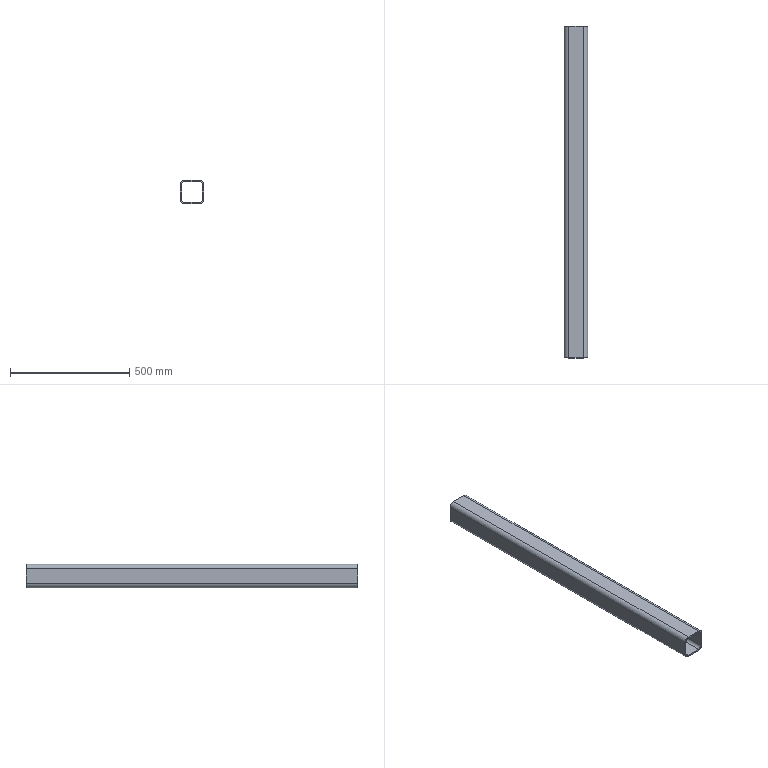Part | SolidWorks | features WeldMemberFeat 1, WeldmentFeature 1 | 1 solid | 18 faces | box 100 x 1393 x 100 mm | volume 2912161 mm3 | plane 10 | cylinder 8 | commonest cylinder face diameters 26.12 x4 38.12 x4
STEP:
#1=CARTESIAN_POINT('',(-50.,0.,30.94));
#2=VERTEX_POINT('',#1);
#3=CARTESIAN_POINT('',(-30.94,0.,50.));
#4=VERTEX_POINT('',#3);
#5=CARTESIAN_POINT('',(-30.94,0.,30.94));
#6=DIRECTION('',(0.,1.,0.));
#7=DIRECTION('',(0.,0.,1.));
#8=AXIS2_PLACEMENT_3D('',#5,#6,#7);
#9=CIRCLE('',#8,19.06);
#10=EDGE_CURVE('',#2,#4,#9,.T.);
#11=ORIENTED_EDGE('',*,*,#10,.T.);
#12=CARTESIAN_POINT('',(-30.94,1393.,50.));
#13=VERTEX_POINT('',#12);
#14=CARTESIAN_POINT('',(-30.94,1393.,50.));
#15=DIRECTION('',(0.,-1.,0.));
#16=VECTOR('',#15,1000.);
#17=LINE('',#14,#16);
#18=EDGE_CURVE('',#13,#4,#17,.T.);
#19=ORIENTED_EDGE('',*,*,#18,.F.);
#20=CARTESIAN_POINT('',(-50.,1393.,30.94));
#21=VERTEX_POINT('',#20);
#22=CARTESIAN_POINT('',(-30.94,1393.,30.94));
#23=DIRECTION('',(0.,1.,0.));
#24=DIRECTION('',(0.,0.,1.));
#25=AXIS2_PLACEMENT_3D('',#22,#23,#24);
#26=CIRCLE('',#25,19.06);
#27=EDGE_CURVE('',#21,#13,#26,.T.);
#28=ORIENTED_EDGE('',*,*,#27,.F.);
#29=CARTESIAN_POINT('',(-50.,1393.,30.94));
#30=DIRECTION('',(0.,-1.,0.));
#31=VECTOR('',#30,1000.);
#32=LINE('',#29,#31);
#33=EDGE_CURVE('',#21,#2,#32,.T.);
#34=ORIENTED_EDGE('',*,*,#33,.T.);
#35=EDGE_LOOP('',(#11,#19,#28,#34));
#36=FACE_OUTER_BOUND('',#35,.T.);
#37=CARTESIAN_POINT('',(-30.94,1393.,30.94));
#38=DIRECTION('',(0.,-1.,0.));
#39=DIRECTION('',(0.,0.,-1.));
#40=AXIS2_PLACEMENT_3D('',#37,#38,#39);
#41=CYLINDRICAL_SURFACE('',#40,19.06);
#42=ADVANCED_FACE('',(#36),#41,.T.);
#43=CARTESIAN_POINT('',(30.94,0.,50.));
#44=VERTEX_POINT('',#43);
#45=CARTESIAN_POINT('',(-30.94,0.,50.));
#46=DIRECTION('',(1.,0.,0.));
#47=VECTOR('',#46,1000.);
#48=LINE('',#45,#47);
#49=EDGE_CURVE('',#4,#44,#48,.T.);
#50=ORIENTED_EDGE('',*,*,#49,.T.);
#51=CARTESIAN_POINT('',(30.94,1393.,50.));
#52=VERTEX_POINT('',#51);
#53=CARTESIAN_POINT('',(30.94,1393.,50.));
#54=DIRECTION('',(0.,-1.,0.));
#55=VECTOR('',#54,1000.);
#56=LINE('',#53,#55);
#57=EDGE_CURVE('',#52,#44,#56,.T.);
#58=ORIENTED_EDGE('',*,*,#57,.F.);
#59=CARTESIAN_POINT('',(-30.94,1393.,50.));
#60=DIRECTION('',(1.,0.,0.));
#61=VECTOR('',#60,1000.);
#62=LINE('',#59,#61);
#63=EDGE_CURVE('',#13,#52,#62,.T.);
#64=ORIENTED_EDGE('',*,*,#63,.F.);
#65=ORIENTED_EDGE('',*,*,#18,.T.);
#66=EDGE_LOOP('',(#50,#58,#64,#65));
#67=FACE_OUTER_BOUND('',#66,.T.);
#68=CARTESIAN_POINT('',(-30.94,1393.,50.));
#69=DIRECTION('',(0.,0.,-1.));
#70=DIRECTION('',(-1.,0.,0.));
#71=AXIS2_PLACEMENT_3D('',#68,#69,#70);
#72=PLANE('',#71);
#73=ADVANCED_FACE('',(#67),#72,.F.);
#74=CARTESIAN_POINT('',(50.,0.,30.94));
#75=VERTEX_POINT('',#74);
#76=CARTESIAN_POINT('',(30.94,0.,30.94));
#77=DIRECTION('',(0.,1.,0.));
#78=DIRECTION('',(0.,0.,1.));
#79=AXIS2_PLACEMENT_3D('',#76,#77,#78);
#80=CIRCLE('',#79,19.06);
#81=EDGE_CURVE('',#44,#75,#80,.T.);
#82=ORIENTED_EDGE('',*,*,#81,.T.);
#83=CARTESIAN_POINT('',(50.,1393.,30.94));
#84=VERTEX_POINT('',#83);
#85=CARTESIAN_POINT('',(50.,1393.,30.94));
#86=DIRECTION('',(0.,-1.,0.));
#87=VECTOR('',#86,1000.);
#88=LINE('',#85,#87);
#89=EDGE_CURVE('',#84,#75,#88,.T.);
#90=ORIENTED_EDGE('',*,*,#89,.F.);
#91=CARTESIAN_POINT('',(30.94,1393.,30.94));
#92=DIRECTION('',(0.,1.,0.));
#93=DIRECTION('',(0.,0.,1.));
#94=AXIS2_PLACEMENT_3D('',#91,#92,#93);
#95=CIRCLE('',#94,19.06);
#96=EDGE_CURVE('',#52,#84,#95,.T.);
#97=ORIENTED_EDGE('',*,*,#96,.F.);
#98=ORIENTED_EDGE('',*,*,#57,.T.);
#99=EDGE_LOOP('',(#82,#90,#97,#98));
#100=FACE_OUTER_BOUND('',#99,.T.);
#101=CARTESIAN_POINT('',(30.94,1393.,30.94));
#102=DIRECTION('',(0.,-1.,0.));
#103=DIRECTION('',(0.,0.,-1.));
#104=AXIS2_PLACEMENT_3D('',#101,#102,#103);
#105=CYLINDRICAL_SURFACE('',#104,19.06);
#106=ADVANCED_FACE('',(#100),#105,.T.);
#107=CARTESIAN_POINT('',(50.,0.,-30.94));
#108=VERTEX_POINT('',#107);
#109=CARTESIAN_POINT('',(50.,0.,-30.94));
#110=DIRECTION('',(0.,0.,-1.));
#111=VECTOR('',#110,1000.);
#112=LINE('',#109,#111);
#113=EDGE_CURVE('',#75,#108,#112,.T.);
#114=ORIENTED_EDGE('',*,*,#113,.T.);
#115=CARTESIAN_POINT('',(50.,1393.,-30.94));
#116=VERTEX_POINT('',#115);
#117=CARTESIAN_POINT('',(50.,1393.,-30.94));
#118=DIRECTION('',(0.,-1.,0.));
#119=VECTOR('',#118,1000.);
#120=LINE('',#117,#119);
#121=EDGE_CURVE('',#116,#108,#120,.T.);
#122=ORIENTED_EDGE('',*,*,#121,.F.);
#123=CARTESIAN_POINT('',(50.,1393.,-30.94));
#124=DIRECTION('',(0.,0.,-1.));
#125=VECTOR('',#124,1000.);
#126=LINE('',#123,#125);
#127=EDGE_CURVE('',#84,#116,#126,.T.);
#128=ORIENTED_EDGE('',*,*,#127,.F.);
#129=ORIENTED_EDGE('',*,*,#89,.T.);
#130=EDGE_LOOP('',(#114,#122,#128,#129));
#131=FACE_OUTER_BOUND('',#130,.T.);
#132=CARTESIAN_POINT('',(50.,1393.,-30.94));
#133=DIRECTION('',(-1.,0.,0.));
#134=DIRECTION('',(0.,0.,1.));
#135=AXIS2_PLACEMENT_3D('',#132,#133,#134);
#136=PLANE('',#135);
#137=ADVANCED_FACE('',(#131),#136,.F.);
#138=CARTESIAN_POINT('',(30.94,0.,-50.));
#139=VERTEX_POINT('',#138);
#140=CARTESIAN_POINT('',(30.94,0.,-30.94));
#141=DIRECTION('',(0.,1.,0.));
#142=DIRECTION('',(0.,0.,1.));
#143=AXIS2_PLACEMENT_3D('',#140,#141,#142);
#144=CIRCLE('',#143,19.06);
#145=EDGE_CURVE('',#108,#139,#144,.T.);
#146=ORIENTED_EDGE('',*,*,#145,.T.);
#147=CARTESIAN_POINT('',(30.94,1393.,-50.));
#148=VERTEX_POINT('',#147);
#149=CARTESIAN_POINT('',(30.94,1393.,-50.));
#150=DIRECTION('',(0.,-1.,0.));
#151=VECTOR('',#150,1000.);
#152=LINE('',#149,#151);
#153=EDGE_CURVE('',#148,#139,#152,.T.);
#154=ORIENTED_EDGE('',*,*,#153,.F.);
#155=CARTESIAN_POINT('',(30.94,1393.,-30.94));
#156=DIRECTION('',(0.,1.,0.));
#157=DIRECTION('',(0.,0.,1.));
#158=AXIS2_PLACEMENT_3D('',#155,#156,#157);
#159=CIRCLE('',#158,19.06);
#160=EDGE_CURVE('',#116,#148,#159,.T.);
#161=ORIENTED_EDGE('',*,*,#160,.F.);
#162=ORIENTED_EDGE('',*,*,#121,.T.);
#163=EDGE_LOOP('',(#146,#154,#161,#162));
#164=FACE_OUTER_BOUND('',#163,.T.);
#165=CARTESIAN_POINT('',(30.94,1393.,-30.94));
#166=DIRECTION('',(0.,-1.,0.));
#167=DIRECTION('',(0.,0.,-1.));
#168=AXIS2_PLACEMENT_3D('',#165,#166,#167);
#169=CYLINDRICAL_SURFACE('',#168,19.06);
#170=ADVANCED_FACE('',(#164),#169,.T.);
#171=CARTESIAN_POINT('',(-30.94,0.,-50.));
#172=VERTEX_POINT('',#171);
#173=CARTESIAN_POINT('',(30.94,0.,-50.));
#174=DIRECTION('',(-1.,0.,0.));
#175=VECTOR('',#174,1000.);
#176=LINE('',#173,#175);
#177=EDGE_CURVE('',#139,#172,#176,.T.);
#178=ORIENTED_EDGE('',*,*,#177,.T.);
#179=CARTESIAN_POINT('',(-30.94,1393.,-50.));
#180=VERTEX_POINT('',#179);
#181=CARTESIAN_POINT('',(-30.94,1393.,-50.));
#182=DIRECTION('',(0.,-1.,0.));
#183=VECTOR('',#182,1000.);
#184=LINE('',#181,#183);
#185=EDGE_CURVE('',#180,#172,#184,.T.);
#186=ORIENTED_EDGE('',*,*,#185,.F.);
#187=CARTESIAN_POINT('',(30.94,1393.,-50.));
#188=DIRECTION('',(-1.,0.,0.));
#189=VECTOR('',#188,1000.);
#190=LINE('',#187,#189);
#191=EDGE_CURVE('',#148,#180,#190,.T.);
#192=ORIENTED_EDGE('',*,*,#191,.F.);
#193=ORIENTED_EDGE('',*,*,#153,.T.);
#194=EDGE_LOOP('',(#178,#186,#192,#193));
#195=FACE_OUTER_BOUND('',#194,.T.);
#196=CARTESIAN_POINT('',(30.94,1393.,-50.));
#197=DIRECTION('',(0.,0.,1.));
#198=DIRECTION('',(1.,0.,0.));
#199=AXIS2_PLACEMENT_3D('',#196,#197,#198);
#200=PLANE('',#199);
#201=ADVANCED_FACE('',(#195),#200,.F.);
#202=CARTESIAN_POINT('',(-50.,0.,-30.94));
#203=VERTEX_POINT('',#202);
#204=CARTESIAN_POINT('',(-30.94,0.,-30.94));
#205=DIRECTION('',(0.,1.,0.));
#206=DIRECTION('',(0.,0.,1.));
#207=AXIS2_PLACEMENT_3D('',#204,#205,#206);
#208=CIRCLE('',#207,19.06);
#209=EDGE_CURVE('',#172,#203,#208,.T.);
#210=ORIENTED_EDGE('',*,*,#209,.T.);
#211=CARTESIAN_POINT('',(-50.,1393.,-30.94));
#212=VERTEX_POINT('',#211);
#213=CARTESIAN_POINT('',(-50.,1393.,-30.94));
#214=DIRECTION('',(0.,-1.,0.));
#215=VECTOR('',#214,1000.);
#216=LINE('',#213,#215);
#217=EDGE_CURVE('',#212,#203,#216,.T.);
#218=ORIENTED_EDGE('',*,*,#217,.F.);
#219=CARTESIAN_POINT('',(-30.94,1393.,-30.94));
#220=DIRECTION('',(0.,1.,0.));
#221=DIRECTION('',(0.,0.,1.));
#222=AXIS2_PLACEMENT_3D('',#219,#220,#221);
#223=CIRCLE('',#222,19.06);
#224=EDGE_CURVE('',#180,#212,#223,.T.);
#225=ORIENTED_EDGE('',*,*,#224,.F.);
#226=ORIENTED_EDGE('',*,*,#185,.T.);
#227=EDGE_LOOP('',(#210,#218,#225,#226));
#228=FACE_OUTER_BOUND('',#227,.T.);
#229=CARTESIAN_POINT('',(-30.94,1393.,-30.94));
#230=DIRECTION('',(0.,-1.,0.));
#231=DIRECTION('',(0.,0.,-1.));
#232=AXIS2_PLACEMENT_3D('',#229,#230,#231);
#233=CYLINDRICAL_SURFACE('',#232,19.06);
#234=ADVANCED_FACE('',(#228),#233,.T.);
#235=CARTESIAN_POINT('',(30.94,0.,44.));
#236=VERTEX_POINT('',#235);
#237=CARTESIAN_POINT('',(44.,0.,30.94));
#238=VERTEX_POINT('',#237);
#239=CARTESIAN_POINT('',(30.94,0.,30.94));
#240=DIRECTION('',(0.,1.,0.));
#241=DIRECTION('',(0.,0.,1.));
#242=AXIS2_PLACEMENT_3D('',#239,#240,#241);
#243=CIRCLE('',#242,13.06);
#244=EDGE_CURVE('',#236,#238,#243,.T.);
#245=ORIENTED_EDGE('',*,*,#244,.F.);
#246=CARTESIAN_POINT('',(30.94,1393.,44.));
#247=VERTEX_POINT('',#246);
#248=CARTESIAN_POINT('',(30.94,1393.,44.));
#249=DIRECTION('',(0.,-1.,0.));
#250=VECTOR('',#249,1000.);
#251=LINE('',#248,#250);
#252=EDGE_CURVE('',#247,#236,#251,.T.);
#253=ORIENTED_EDGE('',*,*,#252,.F.);
#254=CARTESIAN_POINT('',(44.,1393.,30.94));
#255=VERTEX_POINT('',#254);
#256=CARTESIAN_POINT('',(30.94,1393.,30.94));
#257=DIRECTION('',(0.,1.,0.));
#258=DIRECTION('',(0.,0.,1.));
#259=AXIS2_PLACEMENT_3D('',#256,#257,#258);
#260=CIRCLE('',#259,13.06);
#261=EDGE_CURVE('',#247,#255,#260,.T.);
#262=ORIENTED_EDGE('',*,*,#261,.T.);
#263=CARTESIAN_POINT('',(44.,1393.,30.94));
#264=DIRECTION('',(0.,-1.,0.));
#265=VECTOR('',#264,1000.);
#266=LINE('',#263,#265);
#267=EDGE_CURVE('',#255,#238,#266,.T.);
#268=ORIENTED_EDGE('',*,*,#267,.T.);
#269=EDGE_LOOP('',(#245,#253,#262,#268));
#270=FACE_OUTER_BOUND('',#269,.T.);
#271=CARTESIAN_POINT('',(30.94,1393.,30.94));
#272=DIRECTION('',(0.,-1.,0.));
#273=DIRECTION('',(0.,0.,-1.));
#274=AXIS2_PLACEMENT_3D('',#271,#272,#273);
#275=CYLINDRICAL_SURFACE('',#274,13.06);
#276=ADVANCED_FACE('',(#270),#275,.F.);
#277=CARTESIAN_POINT('',(-30.94,0.,44.));
#278=VERTEX_POINT('',#277);
#279=CARTESIAN_POINT('',(-30.94,0.,44.));
#280=DIRECTION('',(1.,0.,0.));
#281=VECTOR('',#280,1000.);
#282=LINE('',#279,#281);
#283=EDGE_CURVE('',#278,#236,#282,.T.);
#284=ORIENTED_EDGE('',*,*,#283,.F.);
#285=CARTESIAN_POINT('',(-30.94,1393.,44.));
#286=VERTEX_POINT('',#285);
#287=CARTESIAN_POINT('',(-30.94,1393.,44.));
#288=DIRECTION('',(0.,-1.,0.));
#289=VECTOR('',#288,1000.);
#290=LINE('',#287,#289);
#291=EDGE_CURVE('',#286,#278,#290,.T.);
#292=ORIENTED_EDGE('',*,*,#291,.F.);
#293=CARTESIAN_POINT('',(-30.94,1393.,44.));
#294=DIRECTION('',(1.,0.,0.));
#295=VECTOR('',#294,1000.);
#296=LINE('',#293,#295);
#297=EDGE_CURVE('',#286,#247,#296,.T.);
#298=ORIENTED_EDGE('',*,*,#297,.T.);
#299=ORIENTED_EDGE('',*,*,#252,.T.);
#300=EDGE_LOOP('',(#284,#292,#298,#299));
#301=FACE_OUTER_BOUND('',#300,.T.);
#302=CARTESIAN_POINT('',(-30.94,1393.,44.));
#303=DIRECTION('',(0.,0.,-1.));
#304=DIRECTION('',(-1.,0.,0.));
#305=AXIS2_PLACEMENT_3D('',#302,#303,#304);
#306=PLANE('',#305);
#307=ADVANCED_FACE('',(#301),#306,.T.);
#308=CARTESIAN_POINT('',(-44.,0.,30.94));
#309=VERTEX_POINT('',#308);
#310=CARTESIAN_POINT('',(-30.94,0.,30.94));
#311=DIRECTION('',(0.,1.,0.));
#312=DIRECTION('',(0.,0.,1.));
#313=AXIS2_PLACEMENT_3D('',#310,#311,#312);
#314=CIRCLE('',#313,13.06);
#315=EDGE_CURVE('',#309,#278,#314,.T.);
#316=ORIENTED_EDGE('',*,*,#315,.F.);
#317=CARTESIAN_POINT('',(-44.,1393.,30.94));
#318=VERTEX_POINT('',#317);
#319=CARTESIAN_POINT('',(-44.,1393.,30.94));
#320=DIRECTION('',(0.,-1.,0.));
#321=VECTOR('',#320,1000.);
#322=LINE('',#319,#321);
#323=EDGE_CURVE('',#318,#309,#322,.T.);
#324=ORIENTED_EDGE('',*,*,#323,.F.);
#325=CARTESIAN_POINT('',(-30.94,1393.,30.94));
#326=DIRECTION('',(0.,1.,0.));
#327=DIRECTION('',(0.,0.,1.));
#328=AXIS2_PLACEMENT_3D('',#325,#326,#327);
#329=CIRCLE('',#328,13.06);
#330=EDGE_CURVE('',#318,#286,#329,.T.);
#331=ORIENTED_EDGE('',*,*,#330,.T.);
#332=ORIENTED_EDGE('',*,*,#291,.T.);
#333=EDGE_LOOP('',(#316,#324,#331,#332));
#334=FACE_OUTER_BOUND('',#333,.T.);
#335=CARTESIAN_POINT('',(-30.94,1393.,30.94));
#336=DIRECTION('',(0.,-1.,0.));
#337=DIRECTION('',(0.,0.,-1.));
#338=AXIS2_PLACEMENT_3D('',#335,#336,#337);
#339=CYLINDRICAL_SURFACE('',#338,13.06);
#340=ADVANCED_FACE('',(#334),#339,.F.);
#341=CARTESIAN_POINT('',(-44.,0.,-30.94));
#342=VERTEX_POINT('',#341);
#343=CARTESIAN_POINT('',(-44.,0.,30.94));
#344=DIRECTION('',(0.,0.,1.));
#345=VECTOR('',#344,1000.);
#346=LINE('',#343,#345);
#347=EDGE_CURVE('',#342,#309,#346,.T.);
#348=ORIENTED_EDGE('',*,*,#347,.F.);
#349=CARTESIAN_POINT('',(-44.,1393.,-30.94));
#350=VERTEX_POINT('',#349);
#351=CARTESIAN_POINT('',(-44.,1393.,-30.94));
#352=DIRECTION('',(0.,-1.,0.));
#353=VECTOR('',#352,1000.);
#354=LINE('',#351,#353);
#355=EDGE_CURVE('',#350,#342,#354,.T.);
#356=ORIENTED_EDGE('',*,*,#355,.F.);
#357=CARTESIAN_POINT('',(-44.,1393.,30.94));
#358=DIRECTION('',(0.,0.,1.));
#359=VECTOR('',#358,1000.);
#360=LINE('',#357,#359);
#361=EDGE_CURVE('',#350,#318,#360,.T.);
#362=ORIENTED_EDGE('',*,*,#361,.T.);
#363=ORIENTED_EDGE('',*,*,#323,.T.);
#364=EDGE_LOOP('',(#348,#356,#362,#363));
#365=FACE_OUTER_BOUND('',#364,.T.);
#366=CARTESIAN_POINT('',(-44.,1393.,30.94));
#367=DIRECTION('',(1.,0.,0.));
#368=DIRECTION('',(0.,0.,-1.));
#369=AXIS2_PLACEMENT_3D('',#366,#367,#368);
#370=PLANE('',#369);
#371=ADVANCED_FACE('',(#365),#370,.T.);
#372=CARTESIAN_POINT('',(-30.94,0.,-44.));
#373=VERTEX_POINT('',#372);
#374=CARTESIAN_POINT('',(-30.94,0.,-30.94));
#375=DIRECTION('',(0.,1.,0.));
#376=DIRECTION('',(0.,0.,1.));
#377=AXIS2_PLACEMENT_3D('',#374,#375,#376);
#378=CIRCLE('',#377,13.06);
#379=EDGE_CURVE('',#373,#342,#378,.T.);
#380=ORIENTED_EDGE('',*,*,#379,.F.);
#381=CARTESIAN_POINT('',(-30.94,1393.,-44.));
#382=VERTEX_POINT('',#381);
#383=CARTESIAN_POINT('',(-30.94,1393.,-44.));
#384=DIRECTION('',(0.,-1.,0.));
#385=VECTOR('',#384,1000.);
#386=LINE('',#383,#385);
#387=EDGE_CURVE('',#382,#373,#386,.T.);
#388=ORIENTED_EDGE('',*,*,#387,.F.);
#389=CARTESIAN_POINT('',(-30.94,1393.,-30.94));
#390=DIRECTION('',(0.,1.,0.));
#391=DIRECTION('',(0.,0.,1.));
#392=AXIS2_PLACEMENT_3D('',#389,#390,#391);
#393=CIRCLE('',#392,13.06);
#394=EDGE_CURVE('',#382,#350,#393,.T.);
#395=ORIENTED_EDGE('',*,*,#394,.T.);
#396=ORIENTED_EDGE('',*,*,#355,.T.);
#397=EDGE_LOOP('',(#380,#388,#395,#396));
#398=FACE_OUTER_BOUND('',#397,.T.);
#399=CARTESIAN_POINT('',(-30.94,1393.,-30.94));
#400=DIRECTION('',(0.,-1.,0.));
#401=DIRECTION('',(0.,0.,-1.));
#402=AXIS2_PLACEMENT_3D('',#399,#400,#401);
#403=CYLINDRICAL_SURFACE('',#402,13.06);
#404=ADVANCED_FACE('',(#398),#403,.F.);
#405=CARTESIAN_POINT('',(30.94,0.,-44.));
#406=VERTEX_POINT('',#405);
#407=CARTESIAN_POINT('',(30.94,0.,-44.));
#408=DIRECTION('',(-1.,0.,0.));
#409=VECTOR('',#408,1000.);
#410=LINE('',#407,#409);
#411=EDGE_CURVE('',#406,#373,#410,.T.);
#412=ORIENTED_EDGE('',*,*,#411,.F.);
#413=CARTESIAN_POINT('',(30.94,1393.,-44.));
#414=VERTEX_POINT('',#413);
#415=CARTESIAN_POINT('',(30.94,1393.,-44.));
#416=DIRECTION('',(0.,-1.,0.));
#417=VECTOR('',#416,1000.);
#418=LINE('',#415,#417);
#419=EDGE_CURVE('',#414,#406,#418,.T.);
#420=ORIENTED_EDGE('',*,*,#419,.F.);
#421=CARTESIAN_POINT('',(30.94,1393.,-44.));
#422=DIRECTION('',(-1.,0.,0.));
#423=VECTOR('',#422,1000.);
#424=LINE('',#421,#423);
#425=EDGE_CURVE('',#414,#382,#424,.T.);
#426=ORIENTED_EDGE('',*,*,#425,.T.);
#427=ORIENTED_EDGE('',*,*,#387,.T.);
#428=EDGE_LOOP('',(#412,#420,#426,#427));
#429=FACE_OUTER_BOUND('',#428,.T.);
#430=CARTESIAN_POINT('',(30.94,1393.,-44.));
#431=DIRECTION('',(0.,0.,1.));
#432=DIRECTION('',(1.,0.,0.));
#433=AXIS2_PLACEMENT_3D('',#430,#431,#432);
#434=PLANE('',#433);
#435=ADVANCED_FACE('',(#429),#434,.T.);
#436=CARTESIAN_POINT('',(44.,0.,-30.94));
#437=VERTEX_POINT('',#436);
#438=CARTESIAN_POINT('',(30.94,0.,-30.94));
#439=DIRECTION('',(0.,1.,0.));
#440=DIRECTION('',(0.,0.,1.));
#441=AXIS2_PLACEMENT_3D('',#438,#439,#440);
#442=CIRCLE('',#441,13.06);
#443=EDGE_CURVE('',#437,#406,#442,.T.);
#444=ORIENTED_EDGE('',*,*,#443,.F.);
#445=CARTESIAN_POINT('',(44.,1393.,-30.94));
#446=VERTEX_POINT('',#445);
#447=CARTESIAN_POINT('',(44.,1393.,-30.94));
#448=DIRECTION('',(0.,-1.,0.));
#449=VECTOR('',#448,1000.);
#450=LINE('',#447,#449);
#451=EDGE_CURVE('',#446,#437,#450,.T.);
#452=ORIENTED_EDGE('',*,*,#451,.F.);
#453=CARTESIAN_POINT('',(30.94,1393.,-30.94));
#454=DIRECTION('',(0.,1.,0.));
#455=DIRECTION('',(0.,0.,1.));
#456=AXIS2_PLACEMENT_3D('',#453,#454,#455);
#457=CIRCLE('',#456,13.06);
#458=EDGE_CURVE('',#446,#414,#457,.T.);
#459=ORIENTED_EDGE('',*,*,#458,.T.);
#460=ORIENTED_EDGE('',*,*,#419,.T.);
#461=EDGE_LOOP('',(#444,#452,#459,#460));
#462=FACE_OUTER_BOUND('',#461,.T.);
#463=CARTESIAN_POINT('',(30.94,1393.,-30.94));
#464=DIRECTION('',(0.,-1.,0.));
#465=DIRECTION('',(0.,0.,-1.));
#466=AXIS2_PLACEMENT_3D('',#463,#464,#465);
#467=CYLINDRICAL_SURFACE('',#466,13.06);
#468=ADVANCED_FACE('',(#462),#467,.F.);
#469=CARTESIAN_POINT('',(44.,0.,-30.94));
#470=DIRECTION('',(0.,0.,-1.));
#471=VECTOR('',#470,1000.);
#472=LINE('',#469,#471);
#473=EDGE_CURVE('',#238,#437,#472,.T.);
#474=ORIENTED_EDGE('',*,*,#473,.F.);
#475=ORIENTED_EDGE('',*,*,#267,.F.);
#476=CARTESIAN_POINT('',(44.,1393.,-30.94));
#477=DIRECTION('',(0.,0.,-1.));
#478=VECTOR('',#477,1000.);
#479=LINE('',#476,#478);
#480=EDGE_CURVE('',#255,#446,#479,.T.);
#481=ORIENTED_EDGE('',*,*,#480,.T.);
#482=ORIENTED_EDGE('',*,*,#451,.T.);
#483=EDGE_LOOP('',(#474,#475,#481,#482));
#484=FACE_OUTER_BOUND('',#483,.T.);
#485=CARTESIAN_POINT('',(44.,1393.,-30.94));
#486=DIRECTION('',(-1.,0.,0.));
#487=DIRECTION('',(0.,0.,1.));
#488=AXIS2_PLACEMENT_3D('',#485,#486,#487);
#489=PLANE('',#488);
#490=ADVANCED_FACE('',(#484),#489,.T.);
#491=CARTESIAN_POINT('',(-50.,0.,30.94));
#492=DIRECTION('',(0.,0.,1.));
#493=VECTOR('',#492,1000.);
#494=LINE('',#491,#493);
#495=EDGE_CURVE('',#203,#2,#494,.T.);
#496=ORIENTED_EDGE('',*,*,#495,.T.);
#497=ORIENTED_EDGE('',*,*,#33,.F.);
#498=CARTESIAN_POINT('',(-50.,1393.,30.94));
#499=DIRECTION('',(0.,0.,1.));
#500=VECTOR('',#499,1000.);
#501=LINE('',#498,#500);
#502=EDGE_CURVE('',#212,#21,#501,.T.);
#503=ORIENTED_EDGE('',*,*,#502,.F.);
#504=ORIENTED_EDGE('',*,*,#217,.T.);
#505=EDGE_LOOP('',(#496,#497,#503,#504));
#506=FACE_OUTER_BOUND('',#505,.T.);
#507=CARTESIAN_POINT('',(-50.,1393.,30.94));
#508=DIRECTION('',(1.,0.,0.));
#509=DIRECTION('',(0.,0.,-1.));
#510=AXIS2_PLACEMENT_3D('',#507,#508,#509);
#511=PLANE('',#510);
#512=ADVANCED_FACE('',(#506),#511,.F.);
#513=ORIENTED_EDGE('',*,*,#261,.F.);
#514=ORIENTED_EDGE('',*,*,#297,.F.);
#515=ORIENTED_EDGE('',*,*,#330,.F.);
#516=ORIENTED_EDGE('',*,*,#361,.F.);
#517=ORIENTED_EDGE('',*,*,#394,.F.);
#518=ORIENTED_EDGE('',*,*,#425,.F.);
#519=ORIENTED_EDGE('',*,*,#458,.F.);
#520=ORIENTED_EDGE('',*,*,#480,.F.);
#521=EDGE_LOOP('',(#513,#514,#515,#516,#517,#518,#519,#520));
#522=FACE_BOUND('',#521,.T.);
#523=ORIENTED_EDGE('',*,*,#27,.T.);
#524=ORIENTED_EDGE('',*,*,#63,.T.);
#525=ORIENTED_EDGE('',*,*,#96,.T.);
#526=ORIENTED_EDGE('',*,*,#127,.T.);
#527=ORIENTED_EDGE('',*,*,#160,.T.);
#528=ORIENTED_EDGE('',*,*,#191,.T.);
#529=ORIENTED_EDGE('',*,*,#224,.T.);
#530=ORIENTED_EDGE('',*,*,#502,.T.);
#531=EDGE_LOOP('',(#523,#524,#525,#526,#527,#528,#529,#530));
#532=FACE_OUTER_BOUND('',#531,.T.);
#533=CARTESIAN_POINT('',(-30.94,1393.,30.94));
#534=DIRECTION('',(0.,1.,0.));
#535=DIRECTION('',(0.,0.,1.));
#536=AXIS2_PLACEMENT_3D('',#533,#534,#535);
#537=PLANE('',#536);
#538=ADVANCED_FACE('',(#522,#532),#537,.T.);
#539=ORIENTED_EDGE('',*,*,#244,.T.);
#540=ORIENTED_EDGE('',*,*,#473,.T.);
#541=ORIENTED_EDGE('',*,*,#443,.T.);
#542=ORIENTED_EDGE('',*,*,#411,.T.);
#543=ORIENTED_EDGE('',*,*,#379,.T.);
#544=ORIENTED_EDGE('',*,*,#347,.T.);
#545=ORIENTED_EDGE('',*,*,#315,.T.);
#546=ORIENTED_EDGE('',*,*,#283,.T.);
#547=EDGE_LOOP('',(#539,#540,#541,#542,#543,#544,#545,#546));
#548=FACE_BOUND('',#547,.T.);
#549=ORIENTED_EDGE('',*,*,#10,.F.);
#550=ORIENTED_EDGE('',*,*,#495,.F.);
#551=ORIENTED_EDGE('',*,*,#209,.F.);
#552=ORIENTED_EDGE('',*,*,#177,.F.);
#553=ORIENTED_EDGE('',*,*,#145,.F.);
#554=ORIENTED_EDGE('',*,*,#113,.F.);
#555=ORIENTED_EDGE('',*,*,#81,.F.);
#556=ORIENTED_EDGE('',*,*,#49,.F.);
#557=EDGE_LOOP('',(#549,#550,#551,#552,#553,#554,#555,#556));
#558=FACE_OUTER_BOUND('',#557,.T.);
#559=CARTESIAN_POINT('',(-30.94,0.,30.94));
#560=DIRECTION('',(0.,1.,0.));
#561=DIRECTION('',(0.,0.,1.));
#562=AXIS2_PLACEMENT_3D('',#559,#560,#561);
#563=PLANE('',#562);
#564=ADVANCED_FACE('',(#548,#558),#563,.F.);
#565=CLOSED_SHELL('',(#42,#73,#106,#137,#170,#201,#234,#276,#307,#340,#371,#404,#435,#468,#490,#512,#538,#564));
#566=MANIFOLD_SOLID_BREP('',#565);
#567=CARTESIAN_POINT('',(0.,0.,0.));
#568=DIRECTION('',(0.,0.,1.));
#569=DIRECTION('',(1.,0.,0.));
#570=AXIS2_PLACEMENT_3D('',#567,#568,#569);
#571=(LENGTH_UNIT()NAMED_UNIT(*)SI_UNIT(.MILLI.,.METRE.));
#572=UNCERTAINTY_MEASURE_WITH_UNIT(LENGTH_MEASURE(0.00001),#571,'','');
#573=(NAMED_UNIT(*)PLANE_ANGLE_UNIT()SI_UNIT($,.RADIAN.));
#574=(NAMED_UNIT(*)SI_UNIT($,.STERADIAN.)SOLID_ANGLE_UNIT());
#575=(GEOMETRIC_REPRESENTATION_CONTEXT(3)GLOBAL_UNCERTAINTY_ASSIGNED_CONTEXT((#572))GLOBAL_UNIT_ASSIGNED_CONTEXT((#571,#573,#574))REPRESENTATION_CONTEXT('',''));
#576=ADVANCED_BREP_SHAPE_REPRESENTATION('',(#566,#570),#575);